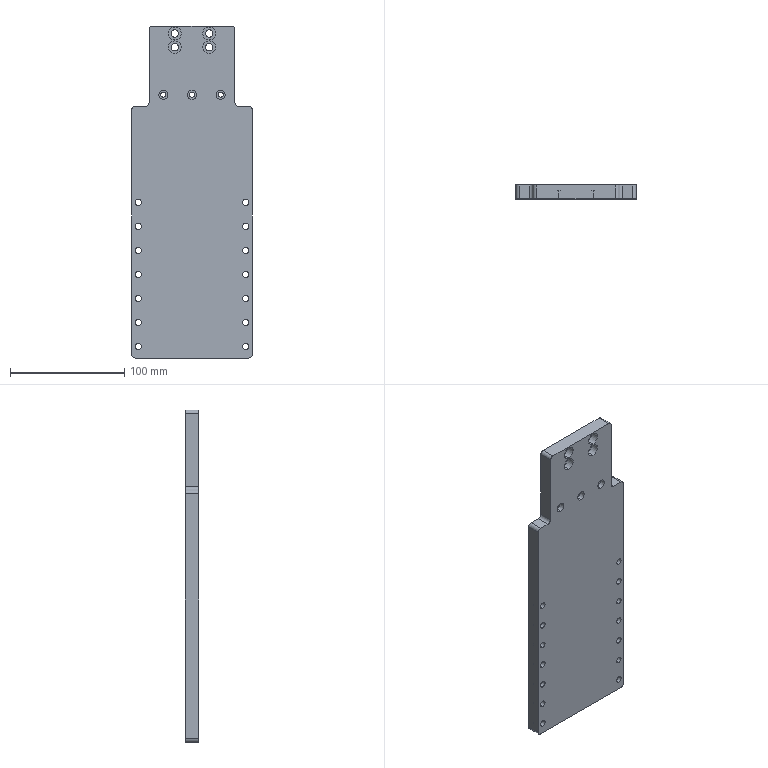Part | STEP file | 1 solid | 179 faces | box 105 x 12 x 290 mm | volume 325340 mm3 | cylinder 120 | plane 31 | cone 28 | commonest cylinder face diameters 5.5 x28 10 x28 3.3 x20 8 x10 6 x8 6.6 x8